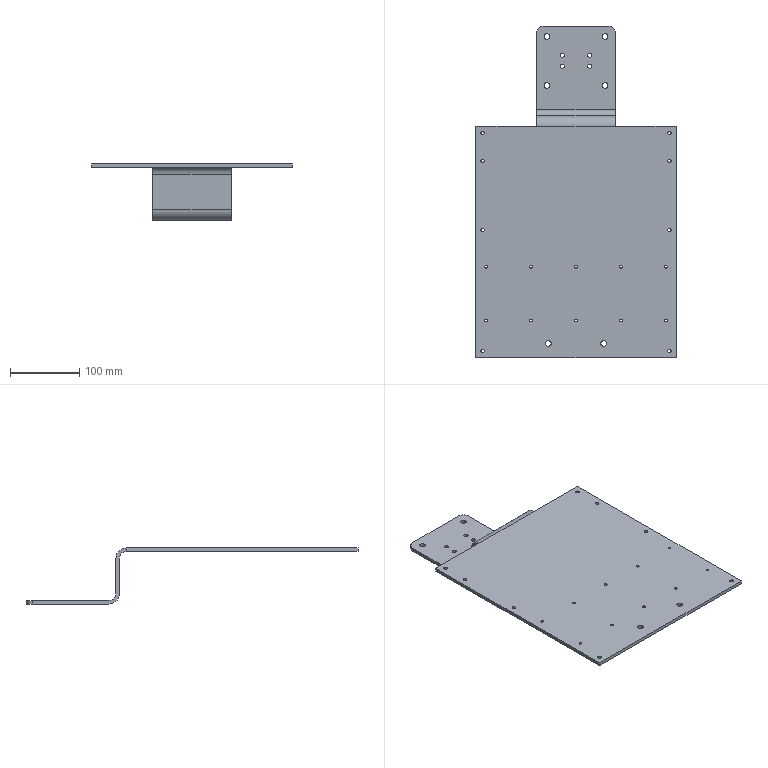Part | SolidWorks | features Cut 5, ICE 4, Fillet 3, Extrusion 1 | 1 solid | 76 faces | box 290 x 480 x 81 mm | volume 601902 mm3 | cylinder 62 | plane 14 | commonest cylinder face diameters 4 x20 5 x16 8 x12 6 x8 20 x4 30 x2